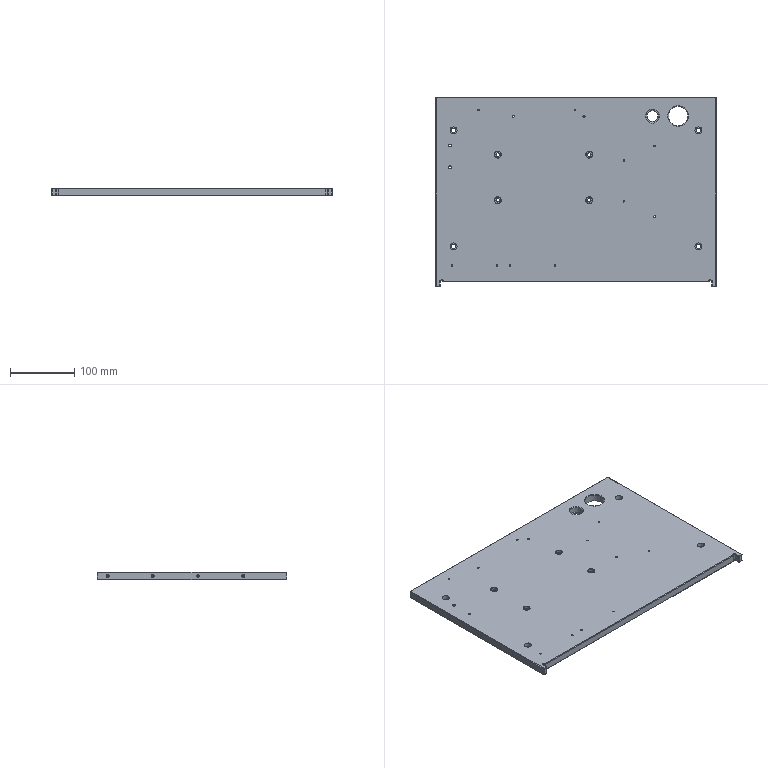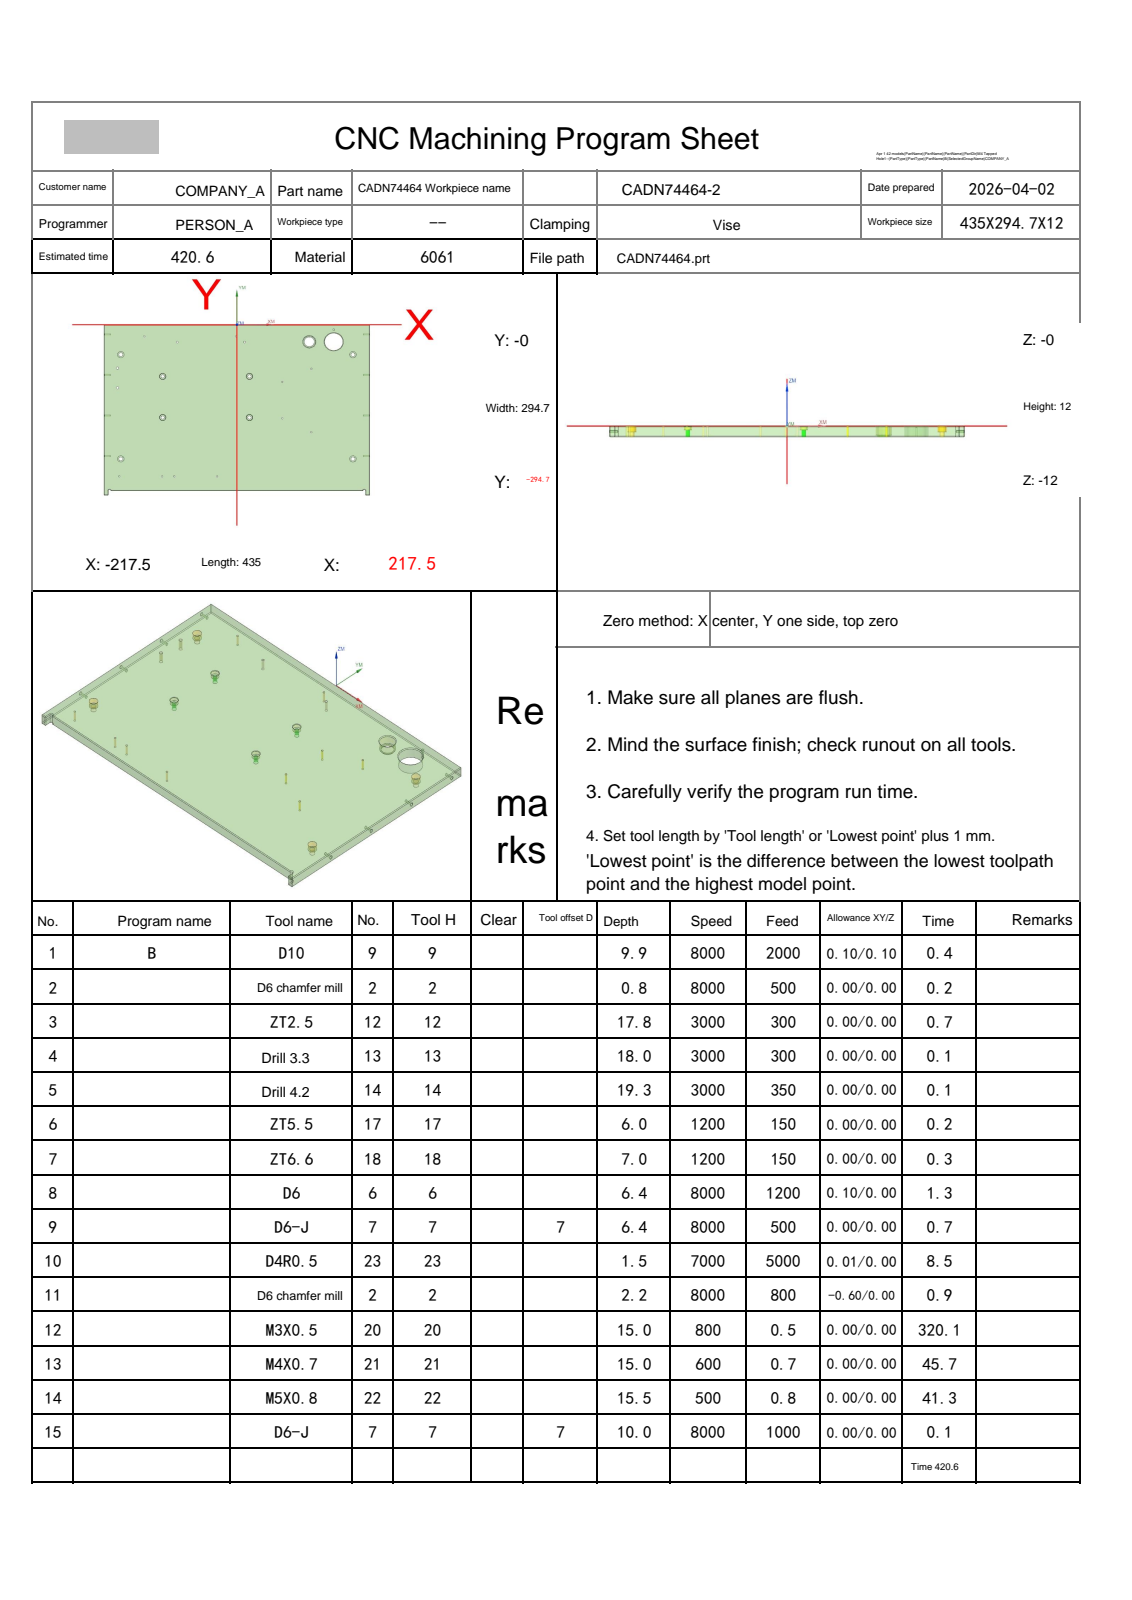NC program | NX | posted by the shop | part box 435 x 294.7 x 12 mm
Lines 1 to 633 of 33933:
%
O0001
(Machine time: 805.26 MIN)
(===Total Tool:13===)
(T9=D10     D=10.  R=0.   D-  H09 Z=-9.9  )
(T2=D6 chamfer mill   D=6.   R=0.   D-  H02 Z=-2.2  )
(T12=ZT2.5  D=2.5  DR_a=118 D-  H12 Z=-17.75)
(T13=Drill 3.3  D=3.3  DR_a=118 D-  H13 Z=-17.99)
(T14=Drill 4.2  D=4.2  DR_a=118 D-  H14 Z=-19.26)
(T17=ZT5.5  D=5.5  DR_a=118 D-  H17 Z=-6.   )
(T18=ZT6.6  D=6.6  DR_a=118 D-  H18 Z=-7.   )
(T6=D6      D=6.   R=0.   D-  H06 Z=-6.4  )
(T7=D6-J    D=6.   R=0.   D7  H07 Z=-10.  )
(T23=D4R0.5 D=4.   R=0.5  D-  H23 Z=-1.5  )
(T20=M3X0.5 D=2.5  DR_a=180 D-  H20 Z=-15.  )
(T21=M4X0.7 D=3.3  DR_a=180 D-  H21 Z=-15.  )
(T22=M5X0.8 D=4.2  DR_a=180 D-  H22 Z=-15.5 )
G80 G90 G17 G49 G40
G91 G28 Z0
M01
N1 T09 M06
(D10  D=10. R=0. H=09 ce=0.10 di=0.10)
G00 G90 G54 X115.203 Y-33.112 M03 S8000
G43 H09 Z20.
M08
Z1.
G01 X115.515 Y-33.424 Z.977 F2000.
X116.67 Y-34.078 Z.907
X117.957 Y-34.4 Z.838
X119.043 Z.781
X120.33 Y-34.078 Z.711
X121.485 Y-33.424 Z.642
X122.424 Y-32.485 Z.572
X123.078 Y-31.33 Z.503
X123.4 Y-30.043 Z.433
Y-28.957 Z.376
X123.078 Y-27.67 Z.307
X122.424 Y-26.515 Z.237
X121.485 Y-25.576 Z.168
X120.33 Y-24.922 Z.098
X119.043 Y-24.6 Z.028
X118.5 Z0.0
G03 X113.6 Y-29.5 Z-.099 I0.0 J-4.9
X118.5 Y-34.4 Z-.198 I4.9 J0.0
X123.4 Y-29.5 Z-.297 I0.0 J4.9
X118.5 Y-24.6 Z-.396 I-4.9 J0.0
X113.6 Y-29.5 Z-.495 I0.0 J-4.9
X118.5 Y-34.4 Z-.594 I4.9 J0.0
X123.4 Y-29.5 Z-.693 I0.0 J4.9
X118.5 Y-24.6 Z-.792 I-4.9 J0.0
X113.6 Y-29.5 Z-.891 I0.0 J-4.9
X118.5 Y-34.4 Z-.99 I4.9 J0.0
X123.4 Y-29.5 Z-1.089 I0.0 J4.9
X118.5 Y-24.6 Z-1.188 I-4.9 J0.0
X113.6 Y-29.5 Z-1.287 I0.0 J-4.9
X118.5 Y-34.4 Z-1.386 I4.9 J0.0
X123.4 Y-29.5 Z-1.485 I0.0 J4.9
X118.5 Y-24.6 Z-1.584 I-4.9 J0.0
X113.6 Y-29.5 Z-1.683 I0.0 J-4.9
X118.5 Y-34.4 Z-1.782 I4.9 J0.0
X123.4 Y-29.5 Z-1.881 I0.0 J4.9
X118.5 Y-24.6 Z-1.98 I-4.9 J0.0
X113.6 Y-29.5 Z-2.079 I0.0 J-4.9
X118.5 Y-34.4 Z-2.178 I4.9 J0.0
X123.4 Y-29.5 Z-2.277 I0.0 J4.9
X118.5 Y-24.6 Z-2.376 I-4.9 J0.0
X113.6 Y-29.5 Z-2.475 I0.0 J-4.9
X118.5 Y-34.4 Z-2.574 I4.9 J0.0
X123.4 Y-29.5 Z-2.673 I0.0 J4.9
X118.5 Y-24.6 Z-2.772 I-4.9 J0.0
X113.6 Y-29.5 Z-2.871 I0.0 J-4.9
X118.5 Y-34.4 Z-2.97 I4.9 J0.0
X123.4 Y-29.5 Z-3.069 I0.0 J4.9
X118.5 Y-24.6 Z-3.168 I-4.9 J0.0
X113.6 Y-29.5 Z-3.267 I0.0 J-4.9
X118.5 Y-34.4 Z-3.366 I4.9 J0.0
X123.4 Y-29.5 Z-3.465 I0.0 J4.9
X118.5 Y-24.6 Z-3.564 I-4.9 J0.0
X113.6 Y-29.5 Z-3.663 I0.0 J-4.9
X118.5 Y-34.4 Z-3.762 I4.9 J0.0
X123.4 Y-29.5 Z-3.861 I0.0 J4.9
X118.5 Y-24.6 Z-3.96 I-4.9 J0.0
X113.6 Y-29.5 Z-4.059 I0.0 J-4.9
X118.5 Y-34.4 Z-4.158 I4.9 J0.0
X123.4 Y-29.5 Z-4.257 I0.0 J4.9
X118.5 Y-24.6 Z-4.356 I-4.9 J0.0
X113.6 Y-29.5 Z-4.455 I0.0 J-4.9
X118.5 Y-34.4 Z-4.554 I4.9 J0.0
X123.4 Y-29.5 Z-4.653 I0.0 J4.9
X118.5 Y-24.6 Z-4.752 I-4.9 J0.0
X113.6 Y-29.5 Z-4.851 I0.0 J-4.9
X118.5 Y-34.4 Z-4.95 I4.9 J0.0
X123.4 Y-29.5 Z-5.049 I0.0 J4.9
X118.5 Y-24.6 Z-5.148 I-4.9 J0.0
X113.6 Y-29.5 Z-5.247 I0.0 J-4.9
X118.5 Y-34.4 Z-5.346 I4.9 J0.0
X123.4 Y-29.5 Z-5.445 I0.0 J4.9
X118.5 Y-24.6 Z-5.544 I-4.9 J0.0
X113.6 Y-29.5 Z-5.643 I0.0 J-4.9
X118.5 Y-34.4 Z-5.742 I4.9 J0.0
X123.4 Y-29.5 Z-5.841 I0.0 J4.9
X118.5 Y-24.6 Z-5.94 I-4.9 J0.0
X113.6 Y-29.5 Z-6.039 I0.0 J-4.9
X118.5 Y-34.4 Z-6.138 I4.9 J0.0
X123.4 Y-29.5 Z-6.237 I0.0 J4.9
X118.5 Y-24.6 Z-6.336 I-4.9 J0.0
X113.6 Y-29.5 Z-6.435 I0.0 J-4.9
X118.5 Y-34.4 Z-6.534 I4.9 J0.0
X123.4 Y-29.5 Z-6.633 I0.0 J4.9
X118.5 Y-24.6 Z-6.732 I-4.9 J0.0
X113.6 Y-29.5 Z-6.831 I0.0 J-4.9
X118.5 Y-34.4 Z-6.93 I4.9 J0.0
X123.4 Y-29.5 Z-7.029 I0.0 J4.9
X118.5 Y-24.6 Z-7.128 I-4.9 J0.0
X113.6 Y-29.5 Z-7.227 I0.0 J-4.9
X118.5 Y-34.4 Z-7.326 I4.9 J0.0
X123.4 Y-29.5 Z-7.425 I0.0 J4.9
X118.5 Y-24.6 Z-7.524 I-4.9 J0.0
X113.6 Y-29.5 Z-7.623 I0.0 J-4.9
X118.5 Y-34.4 Z-7.722 I4.9 J0.0
X123.4 Y-29.5 Z-7.821 I0.0 J4.9
X118.5 Y-24.6 Z-7.92 I-4.9 J0.0
X113.6 Y-29.5 Z-8.019 I0.0 J-4.9
X118.5 Y-34.4 Z-8.118 I4.9 J0.0
X123.4 Y-29.5 Z-8.217 I0.0 J4.9
X118.5 Y-24.6 Z-8.316 I-4.9 J0.0
X113.6 Y-29.5 Z-8.415 I0.0 J-4.9
X118.5 Y-34.4 Z-8.514 I4.9 J0.0
X123.4 Y-29.5 Z-8.613 I0.0 J4.9
X118.5 Y-24.6 Z-8.712 I-4.9 J0.0
X113.6 Y-29.5 Z-8.811 I0.0 J-4.9
X118.5 Y-34.4 Z-8.91 I4.9 J0.0
X123.4 Y-29.5 Z-9.009 I0.0 J4.9
X118.5 Y-24.6 Z-9.108 I-4.9 J0.0
X113.6 Y-29.5 Z-9.207 I0.0 J-4.9
X118.5 Y-34.4 Z-9.306 I4.9 J0.0
X123.4 Y-29.5 Z-9.405 I0.0 J4.9
X118.5 Y-24.6 Z-9.504 I-4.9 J0.0
X113.6 Y-29.5 Z-9.603 I0.0 J-4.9
X118.5 Y-34.4 Z-9.702 I4.9 J0.0
X123.4 Y-29.5 Z-9.801 I0.0 J4.9
X118.5 Y-24.6 Z-9.9 I-4.9 J0.0
X113.6 Y-29.5 I0.0 J-4.9
X118.5 Y-34.4 I4.9 J0.0
X123.4 Y-29.5 I0.0 J4.9
X118.5 Y-24.6 I-4.9 J0.0
X118.1 Y-24.616 I0.0 J-4.9
G01 Z-8.9
G00 Z20.
G91 G28 Z0.0
M05
M09
G91 G28 Z0.0
M01
N2 T02 M06
(D6 chamfer mill  D=6. R=0. H=02 ce=0.00 di=0.10)
G00 G90 G54 X-32.5 Y-261.7 M03 S8000
G43 H02 Z20.
M08
G98 G81 X-32.5 Y-261.7 Z-.8 R1. F500.
X-102.5
X-122.5
X-192.5
X-190. Y-231.696
X-121.425 Y-160.241
Y-89.241
X-195.5 Y-109.
Y-75.
X-190. Y-51.696
X-151.5 Y-20.
X-97.5 Y-30.
X-1.5 Y-20.
X12.5 Y-30.
X118.5 Y-29.5
X190. Y-51.696
X121.901 Y-76.021
X74.218 Y-98.649
X20.575 Y-89.241
Y-160.241
X74.218 Y-161.649
X121.901 Y-185.521
X190. Y-231.696
G80
G00 Z20.
G91 G28 Z0.0
M05
M09
G91 G28 Z0.0
M01
N3 T12 M06
(ZT2.5 D=2.5 DR_a=118 H=12)
G00 G90 G54 X-151.5 Y-20. M03 S3000
G43 H12 Z20.
M08
G98 G83 X-151.5 Y-20. Z-17.751 R1. F300. Q2.
X-1.5
G98 G83 X74.218 Y-98.649 Z-17.751 R1. Q2.
X121.901 Y-76.021
Y-185.521
X74.218 Y-161.649
G98 G83 X-32.5 Y-261.7 Z-17.751 R1. Q2.
X-102.5
X-122.5
X-192.5
G80
G00 Z20.
G91 G28 Z0.0
M05
M09
G91 G28 Z0.0
M01
N4 T13 M06
(Drill 3.3 D=3.3 DR_a=118 H=13)
G00 G90 G54 X-97.5 Y-30. M03 S3000
G43 H13 Z20.
M08
G98 G83 X-97.5 Y-30. Z-17.991 R1. F300. Q2.
X12.5
G80
G00 Z20.
G91 G28 Z0.0
M05
M09
G91 G28 Z0.0
M01
N5 T14 M06
(Drill 4.2 D=4.2 DR_a=118 H=14)
G00 G90 G54 X-195.5 Y-109. M03 S3000
G43 H14 Z20.
M08
G98 G83 X-195.5 Y-109. Z-19.262 R1. F350. Q3.
Y-75.
G80
G00 Z20.
G91 G28 Z0.0
M05
M09
G91 G28 Z0.0
M01
N6 T17 M06
(ZT5.5 D=5.5 DR_a=118 H=17)
G00 G90 G54 X-121.425 Y-89.241 M03 S1200
G43 H17 Z20.
M08
G98 G83 X-121.425 Y-89.241 Z-6. R1. F150. Q2.
Y-160.241
X20.575
Y-89.241
G80
G00 Z20.
G91 G28 Z0.0
M05
M09
G91 G28 Z0.0
M01
N7 T18 M06
(ZT6.6 D=6.6 DR_a=118 H=18)
G00 G90 G54 X-190. Y-231.696 M03 S1200
G43 H18 Z20.
M08
G98 G83 X-190. Y-231.696 Z-7. R1. F150. Q2.
Y-51.696
X190.
Y-231.696
G80
G00 Z20.
G91 G28 Z0.0
M05
M09
G91 G28 Z0.0
M01
N8 T06 M06
(D6  D=6. R=0. H=06 ce=0.10 di=0.00)
G00 G90 G54 X-121.425 Y-89.241 M03 S8000
G43 H06 Z20.
M08
Z.5
G03 X-120.475 Y-90.191 I.95 J0.0 F1200.
X-119.525 Y-89.241 I0.0 J.95
X-119.525 Y-89.241 Z0.0 I-1.9 J0.0
X-119.525 Y-89.241 Z-.5 I-1.9 J0.0
X-119.525 Y-89.241 Z-1. I-1.9 J0.0
X-119.525 Y-89.241 Z-1.5 I-1.9 J0.0
X-119.525 Y-89.241 Z-2. I-1.9 J0.0
X-119.525 Y-89.241 Z-2.5 I-1.9 J0.0
X-119.525 Y-89.241 Z-3. I-1.9 J0.0
X-119.525 Y-89.241 Z-3.5 I-1.9 J0.0
X-119.525 Y-89.241 Z-4. I-1.9 J0.0
X-122.962 Y-88.124 Z-4.2 I-1.9 J0.0
X-123.325 Y-89.241 I1.537 J-1.117
X-121.425 Y-91.141 I1.9 J0.0
X-119.525 Y-89.241 I0.0 J1.9
X-121.425 Y-87.341 I-1.9 J0.0
X-122.962 Y-88.124 I0.0 J-1.9
X-123.144 Y-88.682 I.769 J-.558
X-122.194 Y-89.632 I.95 J0.0
X-121.425 Y-89.241 I0.0 J.95
G00 Z20.
Y-160.241
Z.5
G03 X-120.475 Y-161.191 I.95 J0.0
X-119.525 Y-160.241 I0.0 J.95
X-119.525 Y-160.241 Z0.0 I-1.9 J0.0
X-119.525 Y-160.241 Z-.5 I-1.9 J0.0
X-119.525 Y-160.241 Z-1. I-1.9 J0.0
X-119.525 Y-160.241 Z-1.5 I-1.9 J0.0
X-119.525 Y-160.241 Z-2. I-1.9 J0.0
X-119.525 Y-160.241 Z-2.5 I-1.9 J0.0
X-119.525 Y-160.241 Z-3. I-1.9 J0.0
X-119.525 Y-160.241 Z-3.5 I-1.9 J0.0
X-119.525 Y-160.241 Z-4. I-1.9 J0.0
X-122.962 Y-159.124 Z-4.2 I-1.9 J0.0
X-123.325 Y-160.241 I1.537 J-1.117
X-121.425 Y-162.141 I1.9 J0.0
X-119.525 Y-160.241 I0.0 J1.9
X-121.425 Y-158.341 I-1.9 J0.0
X-122.962 Y-159.124 I0.0 J-1.9
X-123.144 Y-159.682 I.769 J-.558
X-122.194 Y-160.632 I.95 J0.0
X-121.425 Y-160.241 I0.0 J.95
G00 Z20.
X20.575
Z.5
G03 X21.525 Y-161.191 I.95 J0.0
X22.475 Y-160.241 I0.0 J.95
X22.475 Y-160.241 Z0.0 I-1.9 J0.0
X22.475 Y-160.241 Z-.5 I-1.9 J0.0
X22.475 Y-160.241 Z-1. I-1.9 J0.0
X22.475 Y-160.241 Z-1.5 I-1.9 J0.0
X22.475 Y-160.241 Z-2. I-1.9 J0.0
X22.475 Y-160.241 Z-2.5 I-1.9 J0.0
X22.475 Y-160.241 Z-3. I-1.9 J0.0
X22.475 Y-160.241 Z-3.5 I-1.9 J0.0
X22.475 Y-160.241 Z-4. I-1.9 J0.0
X19.038 Y-159.124 Z-4.2 I-1.9 J0.0
X18.675 Y-160.241 I1.537 J-1.117
X20.575 Y-162.141 I1.9 J0.0
X22.475 Y-160.241 I0.0 J1.9
X20.575 Y-158.341 I-1.9 J0.0
X19.038 Y-159.124 I0.0 J-1.9
X18.856 Y-159.682 I.769 J-.558
X19.806 Y-160.632 I.95 J0.0
X20.575 Y-160.241 I0.0 J.95
G00 Z20.
Y-89.241
Z.5
G03 X21.525 Y-90.191 I.95 J0.0
X22.475 Y-89.241 I0.0 J.95
X22.475 Y-89.241 Z0.0 I-1.9 J0.0
X22.475 Y-89.241 Z-.5 I-1.9 J0.0
X22.475 Y-89.241 Z-1. I-1.9 J0.0
X22.475 Y-89.241 Z-1.5 I-1.9 J0.0
X22.475 Y-89.241 Z-2. I-1.9 J0.0
X22.475 Y-89.241 Z-2.5 I-1.9 J0.0
X22.475 Y-89.241 Z-3. I-1.9 J0.0
X22.475 Y-89.241 Z-3.5 I-1.9 J0.0
X22.475 Y-89.241 Z-4. I-1.9 J0.0
X19.038 Y-88.124 Z-4.2 I-1.9 J0.0
X18.675 Y-89.241 I1.537 J-1.117
X20.575 Y-91.141 I1.9 J0.0
X22.475 Y-89.241 I0.0 J1.9
X20.575 Y-87.341 I-1.9 J0.0
X19.038 Y-88.124 I0.0 J-1.9
X18.856 Y-88.682 I.769 J-.558
X19.806 Y-89.632 I.95 J0.0
X20.575 Y-89.241 I0.0 J.95
G00 Z20.
G00 G90 X-190. Y-231.696 M03 S8000
Z20.
Z.5
G03 X-188.8 Y-232.896 I1.2 J0.0 F1200.
X-187.6 Y-231.696 I0.0 J1.2
X-187.6 Y-231.696 Z0.0 I-2.4 J0.0
X-187.6 Y-231.696 Z-.5 I-2.4 J0.0
X-187.6 Y-231.696 Z-1. I-2.4 J0.0
X-187.6 Y-231.696 Z-1.5 I-2.4 J0.0
X-187.6 Y-231.696 Z-2. I-2.4 J0.0
X-187.6 Y-231.696 Z-2.5 I-2.4 J0.0
X-187.6 Y-231.696 Z-3. I-2.4 J0.0
X-187.6 Y-231.696 Z-3.5 I-2.4 J0.0
X-187.6 Y-231.696 Z-4. I-2.4 J0.0
X-187.6 Y-231.696 Z-4.5 I-2.4 J0.0
X-187.6 Y-231.696 Z-5. I-2.4 J0.0
X-187.6 Y-231.696 Z-5.5 I-2.4 J0.0
X-187.6 Y-231.696 Z-6. I-2.4 J0.0
X-189.258 Y-233.979 Z-6.4 I-2.4 J0.0
X-187.6 Y-231.696 I-.742 J2.283
X-190. Y-229.296 I-2.4 J0.0
X-192.4 Y-231.696 I0.0 J-2.4
X-190. Y-234.096 I2.4 J0.0
X-189.258 Y-233.979 I0.0 J2.4
X-188.429 Y-232.837 I-.371 J1.141
X-189.629 Y-231.637 I-1.2 J0.0
X-190. Y-231.696 I0.0 J-1.2
G00 Z20.
Y-51.696
Z.5
G03 X-188.8 Y-52.896 I1.2 J0.0
X-187.6 Y-51.696 I0.0 J1.2
X-187.6 Y-51.696 Z0.0 I-2.4 J0.0
X-187.6 Y-51.696 Z-.5 I-2.4 J0.0
X-187.6 Y-51.696 Z-1. I-2.4 J0.0
X-187.6 Y-51.696 Z-1.5 I-2.4 J0.0
X-187.6 Y-51.696 Z-2. I-2.4 J0.0
X-187.6 Y-51.696 Z-2.5 I-2.4 J0.0
X-187.6 Y-51.696 Z-3. I-2.4 J0.0
X-187.6 Y-51.696 Z-3.5 I-2.4 J0.0
X-187.6 Y-51.696 Z-4. I-2.4 J0.0
X-187.6 Y-51.696 Z-4.5 I-2.4 J0.0
X-187.6 Y-51.696 Z-5. I-2.4 J0.0
X-187.6 Y-51.696 Z-5.5 I-2.4 J0.0
X-187.6 Y-51.696 Z-6. I-2.4 J0.0
X-189.258 Y-53.979 Z-6.4 I-2.4 J0.0
X-187.6 Y-51.696 I-.742 J2.283
X-190. Y-49.296 I-2.4 J0.0
X-192.4 Y-51.696 I0.0 J-2.4
X-190. Y-54.096 I2.4 J0.0
X-189.258 Y-53.979 I0.0 J2.4
X-188.429 Y-52.837 I-.371 J1.141
X-189.629 Y-51.637 I-1.2 J0.0
X-190. Y-51.696 I0.0 J-1.2
G00 Z20.
X190.
Z.5
G03 X191.2 Y-52.896 I1.2 J0.0
X192.4 Y-51.696 I0.0 J1.2
X192.4 Y-51.696 Z0.0 I-2.4 J0.0
X192.4 Y-51.696 Z-.5 I-2.4 J0.0
X192.4 Y-51.696 Z-1. I-2.4 J0.0
X192.4 Y-51.696 Z-1.5 I-2.4 J0.0
X192.4 Y-51.696 Z-2. I-2.4 J0.0
X192.4 Y-51.696 Z-2.5 I-2.4 J0.0
X192.4 Y-51.696 Z-3. I-2.4 J0.0
X192.4 Y-51.696 Z-3.5 I-2.4 J0.0
X192.4 Y-51.696 Z-4. I-2.4 J0.0
X192.4 Y-51.696 Z-4.5 I-2.4 J0.0
X192.4 Y-51.696 Z-5. I-2.4 J0.0
X192.4 Y-51.696 Z-5.5 I-2.4 J0.0
X192.4 Y-51.696 Z-6. I-2.4 J0.0
X190.742 Y-53.979 Z-6.4 I-2.4 J0.0
X192.4 Y-51.696 I-.742 J2.283
X190. Y-49.296 I-2.4 J0.0
X187.6 Y-51.696 I0.0 J-2.4
X190. Y-54.096 I2.4 J0.0
X190.742 Y-53.979 I0.0 J2.4
X191.571 Y-52.837 I-.371 J1.141
X190.371 Y-51.637 I-1.2 J0.0
X190. Y-51.696 I0.0 J-1.2
G00 Z20.
Y-231.696
Z.5
G03 X191.2 Y-232.896 I1.2 J0.0
X192.4 Y-231.696 I0.0 J1.2
X192.4 Y-231.696 Z0.0 I-2.4 J0.0
X192.4 Y-231.696 Z-.5 I-2.4 J0.0
X192.4 Y-231.696 Z-1. I-2.4 J0.0
X192.4 Y-231.696 Z-1.5 I-2.4 J0.0
X192.4 Y-231.696 Z-2. I-2.4 J0.0
X192.4 Y-231.696 Z-2.5 I-2.4 J0.0
X192.4 Y-231.696 Z-3. I-2.4 J0.0
X192.4 Y-231.696 Z-3.5 I-2.4 J0.0
X192.4 Y-231.696 Z-4. I-2.4 J0.0
X192.4 Y-231.696 Z-4.5 I-2.4 J0.0
X192.4 Y-231.696 Z-5. I-2.4 J0.0
X192.4 Y-231.696 Z-5.5 I-2.4 J0.0
X192.4 Y-231.696 Z-6. I-2.4 J0.0
X190.742 Y-233.979 Z-6.4 I-2.4 J0.0
X192.4 Y-231.696 I-.742 J2.283
X190. Y-229.296 I-2.4 J0.0
X187.6 Y-231.696 I0.0 J-2.4
X190. Y-234.096 I2.4 J0.0
X190.742 Y-233.979 I0.0 J2.4
X191.571 Y-232.837 I-.371 J1.141
X190.371 Y-231.637 I-1.2 J0.0
X190. Y-231.696 I0.0 J-1.2
G00 Z20.
G91 G28 Z0.0
M05
M09
G91 G28 Z0.0
M01
N9 T07 M06
(D6-J  D=6. R=0. H=07 ce=0.00 di=0.00)
G00 G90 G54 X-121.425 Y-89.241 M03 S8000
G43 H07 Z20.
M08
Z0.0
G41 D07
G01 X-121.386 Y-89.437 F500.
G03 X-120.415 Y-90.231 I.97 J.196
X-119.425 Y-89.241 I0.0 J.99
X-120.353 Y-90.929 Z-4.2 I-2. J0.0
X-119.425 Y-89.241 I-1.072 J1.689
X-121.425 Y-87.241 I-2. J0.0
X-123.425 Y-89.241 I0.0 J-2.
X-121.425 Y-91.241 I2. J0.0
X-120.353 Y-90.929 I0.0 J2.
X-119.894 Y-90.094 I-.53 J.836
X-120.884 Y-89.104 I-.99 J0.0
X-121.238 Y-89.169 I0.0 J-.99
G01 G40 X-121.425 Y-89.241
G00 Z20.
Y-160.241
Z0.0
G41 D07
G01 X-121.386 Y-160.437
G03 X-120.415 Y-161.231 I.97 J.196
X-119.425 Y-160.241 I0.0 J.99
X-120.353 Y-161.929 Z-4.2 I-2. J0.0
X-119.425 Y-160.241 I-1.072 J1.689
X-121.425 Y-158.241 I-2. J0.0
X-123.425 Y-160.241 I0.0 J-2.
X-121.425 Y-162.241 I2. J0.0
X-120.353 Y-161.929 I0.0 J2.
X-119.894 Y-161.094 I-.53 J.836
X-120.884 Y-160.104 I-.99 J0.0
X-121.238 Y-160.169 I0.0 J-.99
G01 G40 X-121.425 Y-160.241
G00 Z20.
X20.575
Z0.0
G41 D07
G01 X20.614 Y-160.437
G03 X21.585 Y-161.231 I.97 J.196
X22.575 Y-160.241 I0.0 J.99
X21.646 Y-161.929 Z-4.2 I-2. J0.0
X22.575 Y-160.241 I-1.072 J1.689
X20.575 Y-158.241 I-2. J0.0
X18.575 Y-160.241 I0.0 J-2.
X20.575 Y-162.241 I2. J0.0
X21.646 Y-161.929 I0.0 J2.
X22.106 Y-161.094 I-.53 J.836
X21.116 Y-160.104 I-.99 J0.0
X20.762 Y-160.169 I0.0 J-.99
G01 G40 X20.575 Y-160.241
G00 Z20.
Y-89.241
Z0.0
G41 D07
G01 X20.614 Y-89.437
G03 X21.585 Y-90.231 I.97 J.196
X22.575 Y-89.241 I0.0 J.99
X21.646 Y-90.929 Z-4.2 I-2. J0.0
X22.575 Y-89.241 I-1.072 J1.689
X20.575 Y-87.241 I-2. J0.0
X18.575 Y-89.241 I0.0 J-2.
X20.575 Y-91.241 I2. J0.0
X21.646 Y-90.929 I0.0 J2.
X22.106 Y-90.094 I-.53 J.836
X21.116 Y-89.104 I-.99 J0.0
X20.762 Y-89.169 I0.0 J-.99
G01 G40 X20.575 Y-89.241
G00 Z20.
G00 G90 X-190. Y-231.696 M03 S8000
Z20.
Z0.0
G41 D07
G01 X-189.968 Y-231.894 F500.
G03 X-188.742 Y-232.938 I1.226 J.197
X-187.5 Y-231.696 I0.0 J1.242
X-187.5 Y-231.696 Z-5. I-2.5 J0.0
X-190.468 Y-229.24 Z-6.4 I-2.5 J0.0
X-192.5 Y-231.696 I.468 J-2.456
X-190. Y-234.196 I2.5 J0.0
X-187.5 Y-231.696 I0.0 J2.5
X-190. Y-229.196 I-2.5 J0.0
X-190.468 Y-229.24 I0.0 J-2.5
X-191.478 Y-230.46 I.233 J-1.22
X-190.236 Y-231.702 I1.242 J0.0
G01 X-190.2
G40 X-190. Y-231.696
G00 Z20.
Y-51.696
Z0.0
G41 D07
G01 X-189.968 Y-51.894
G03 X-188.742 Y-52.938 I1.226 J.197
X-187.5 Y-51.696 I0.0 J1.242
X-187.5 Y-51.696 Z-5. I-2.5 J0.0
X-190.468 Y-49.24 Z-6.4 I-2.5 J0.0
X-192.5 Y-51.696 I.468 J-2.456
X-190. Y-54.196 I2.5 J0.0
X-187.5 Y-51.696 I0.0 J2.5
X-190. Y-49.196 I-2.5 J0.0
X-190.468 Y-49.24 I0.0 J-2.5
X-191.478 Y-50.46 I.233 J-1.22
X-190.236 Y-51.702 I1.242 J0.0
G01 X-190.2
G40 X-190. Y-51.696
G00 Z20.
X190.
Z0.0
G41 D07
G01 X190.032 Y-51.894
G03 X191.258 Y-52.938 I1.226 J.197
X192.5 Y-51.696 I0.0 J1.242
X192.5 Y-51.696 Z-5. I-2.5 J0.0
X189.532 Y-49.24 Z-6.4 I-2.5 J0.0
X187.5 Y-51.696 I.468 J-2.456
X190. Y-54.196 I2.5 J0.0
X192.5 Y-51.696 I0.0 J2.5
X190. Y-49.196 I-2.5 J0.0
X189.532 Y-49.24 I0.0 J-2.5
X188.522 Y-50.46 I.233 J-1.22
X189.764 Y-51.702 I1.242 J0.0
G01 X189.8
G40 X190. Y-51.696
G00 Z20.
Y-231.696
Z0.0
G41 D07
G01 X190.032 Y-231.894
G03 X191.258 Y-232.938 I1.226 J.197
X192.5 Y-231.696 I0.0 J1.242
X192.5 Y-231.696 Z-5. I-2.5 J0.0
X189.532 Y-229.24 Z-6.4 I-2.5 J0.0
X187.5 Y-231.696 I.468 J-2.456
X190. Y-234.196 I2.5 J0.0
X192.5 Y-231.696 I0.0 J2.5
X190. Y-229.196 I-2.5 J0.0
X189.532 Y-229.24 I0.0 J-2.5
X188.522 Y-230.46 I.233 J-1.22
X189.764 Y-231.702 I1.242 J0.0
G01 X189.8
G40 X190. Y-231.696
G00 Z20.
G91 G28 Z0.0
M05
M09
G91 G28 Z0.0
M01